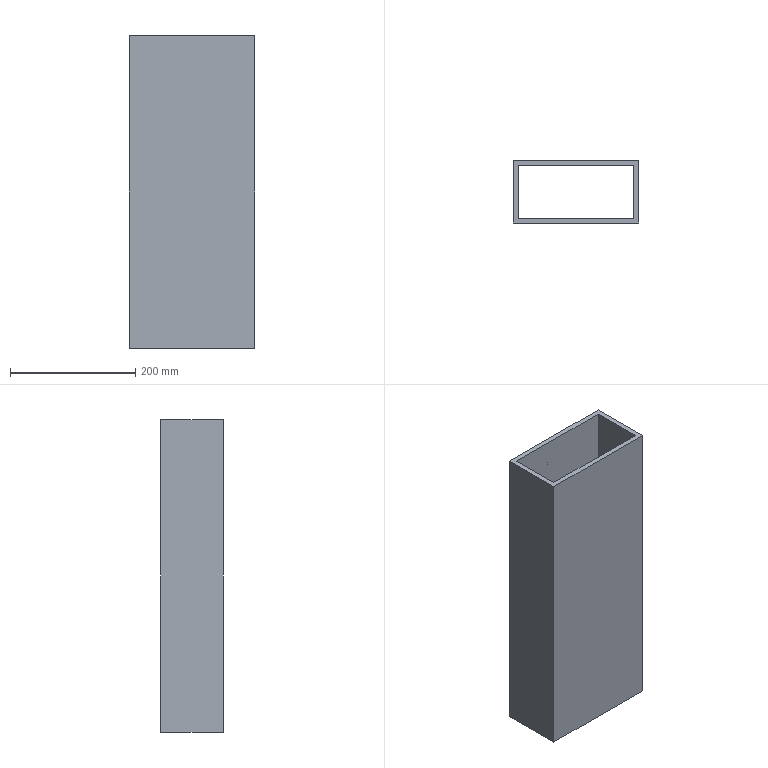Part | SolidWorks | features BaseBody 1 | 1 solid | 34 faces | box 200 x 100 x 500 mm | volume 2270906 mm3 | plane 18 | cylinder 16 | commonest cylinder face diameters 5.3 x16
STEP:
#1=CARTESIAN_POINT('',(20.,43.8,207.35));
#2=VERTEX_POINT('',#1);
#3=CARTESIAN_POINT('',(20.,43.8,212.65));
#4=VERTEX_POINT('',#3);
#5=CARTESIAN_POINT('',(20.,43.8,210.));
#6=DIRECTION('',(0.,1.,0.));
#7=DIRECTION('',(0.,0.,1.));
#8=AXIS2_PLACEMENT_3D('',#5,#6,#7);
#9=CIRCLE('',#8,2.65);
#10=EDGE_CURVE('',#2,#4,#9,.T.);
#11=ORIENTED_EDGE('',*,*,#10,.F.);
#12=CARTESIAN_POINT('',(20.,50.,207.35));
#13=VERTEX_POINT('',#12);
#14=CARTESIAN_POINT('',(20.,43.8,207.35));
#15=DIRECTION('',(0.,1.,0.));
#16=VECTOR('',#15,1000.);
#17=LINE('',#14,#16);
#18=EDGE_CURVE('',#2,#13,#17,.T.);
#19=ORIENTED_EDGE('',*,*,#18,.T.);
#20=CARTESIAN_POINT('',(20.,50.,212.65));
#21=VERTEX_POINT('',#20);
#22=CARTESIAN_POINT('',(20.,50.,210.));
#23=DIRECTION('',(0.,-1.,0.));
#24=DIRECTION('',(0.,0.,1.));
#25=AXIS2_PLACEMENT_3D('',#22,#23,#24);
#26=CIRCLE('',#25,2.65);
#27=EDGE_CURVE('',#21,#13,#26,.T.);
#28=ORIENTED_EDGE('',*,*,#27,.F.);
#29=CARTESIAN_POINT('',(20.,43.8,212.65));
#30=DIRECTION('',(0.,1.,0.));
#31=VECTOR('',#30,1000.);
#32=LINE('',#29,#31);
#33=EDGE_CURVE('',#4,#21,#32,.T.);
#34=ORIENTED_EDGE('',*,*,#33,.F.);
#35=EDGE_LOOP('',(#11,#19,#28,#34));
#36=FACE_OUTER_BOUND('',#35,.T.);
#37=CARTESIAN_POINT('',(20.,43.8,210.));
#38=DIRECTION('',(0.,1.,0.));
#39=DIRECTION('',(0.,0.,1.));
#40=AXIS2_PLACEMENT_3D('',#37,#38,#39);
#41=CYLINDRICAL_SURFACE('',#40,2.65);
#42=ADVANCED_FACE('',(#36),#41,.F.);
#43=CARTESIAN_POINT('',(20.,43.8,87.35));
#44=VERTEX_POINT('',#43);
#45=CARTESIAN_POINT('',(20.,43.8,92.65));
#46=VERTEX_POINT('',#45);
#47=CARTESIAN_POINT('',(20.,43.8,90.));
#48=DIRECTION('',(0.,1.,0.));
#49=DIRECTION('',(0.,0.,1.));
#50=AXIS2_PLACEMENT_3D('',#47,#48,#49);
#51=CIRCLE('',#50,2.65);
#52=EDGE_CURVE('',#44,#46,#51,.T.);
#53=ORIENTED_EDGE('',*,*,#52,.F.);
#54=CARTESIAN_POINT('',(20.,50.,87.35));
#55=VERTEX_POINT('',#54);
#56=CARTESIAN_POINT('',(20.,43.8,87.35));
#57=DIRECTION('',(0.,1.,0.));
#58=VECTOR('',#57,1000.);
#59=LINE('',#56,#58);
#60=EDGE_CURVE('',#44,#55,#59,.T.);
#61=ORIENTED_EDGE('',*,*,#60,.T.);
#62=CARTESIAN_POINT('',(20.,50.,92.65));
#63=VERTEX_POINT('',#62);
#64=CARTESIAN_POINT('',(20.,50.,90.));
#65=DIRECTION('',(0.,-1.,0.));
#66=DIRECTION('',(0.,0.,1.));
#67=AXIS2_PLACEMENT_3D('',#64,#65,#66);
#68=CIRCLE('',#67,2.65);
#69=EDGE_CURVE('',#63,#55,#68,.T.);
#70=ORIENTED_EDGE('',*,*,#69,.F.);
#71=CARTESIAN_POINT('',(20.,43.8,92.65));
#72=DIRECTION('',(0.,1.,0.));
#73=VECTOR('',#72,1000.);
#74=LINE('',#71,#73);
#75=EDGE_CURVE('',#46,#63,#74,.T.);
#76=ORIENTED_EDGE('',*,*,#75,.F.);
#77=EDGE_LOOP('',(#53,#61,#70,#76));
#78=FACE_OUTER_BOUND('',#77,.T.);
#79=CARTESIAN_POINT('',(20.,43.8,90.));
#80=DIRECTION('',(0.,1.,0.));
#81=DIRECTION('',(0.,0.,1.));
#82=AXIS2_PLACEMENT_3D('',#79,#80,#81);
#83=CYLINDRICAL_SURFACE('',#82,2.65);
#84=ADVANCED_FACE('',(#78),#83,.F.);
#85=CARTESIAN_POINT('',(20.,43.8,-32.65));
#86=VERTEX_POINT('',#85);
#87=CARTESIAN_POINT('',(20.,43.8,-27.35));
#88=VERTEX_POINT('',#87);
#89=CARTESIAN_POINT('',(20.,43.8,-30.));
#90=DIRECTION('',(0.,1.,0.));
#91=DIRECTION('',(0.,0.,1.));
#92=AXIS2_PLACEMENT_3D('',#89,#90,#91);
#93=CIRCLE('',#92,2.65);
#94=EDGE_CURVE('',#86,#88,#93,.T.);
#95=ORIENTED_EDGE('',*,*,#94,.F.);
#96=CARTESIAN_POINT('',(20.,50.,-32.65));
#97=VERTEX_POINT('',#96);
#98=CARTESIAN_POINT('',(20.,43.8,-32.65));
#99=DIRECTION('',(0.,1.,0.));
#100=VECTOR('',#99,1000.);
#101=LINE('',#98,#100);
#102=EDGE_CURVE('',#86,#97,#101,.T.);
#103=ORIENTED_EDGE('',*,*,#102,.T.);
#104=CARTESIAN_POINT('',(20.,50.,-27.35));
#105=VERTEX_POINT('',#104);
#106=CARTESIAN_POINT('',(20.,50.,-30.));
#107=DIRECTION('',(0.,-1.,0.));
#108=DIRECTION('',(0.,0.,1.));
#109=AXIS2_PLACEMENT_3D('',#106,#107,#108);
#110=CIRCLE('',#109,2.65);
#111=EDGE_CURVE('',#105,#97,#110,.T.);
#112=ORIENTED_EDGE('',*,*,#111,.F.);
#113=CARTESIAN_POINT('',(20.,43.8,-27.35));
#114=DIRECTION('',(0.,1.,0.));
#115=VECTOR('',#114,1000.);
#116=LINE('',#113,#115);
#117=EDGE_CURVE('',#88,#105,#116,.T.);
#118=ORIENTED_EDGE('',*,*,#117,.F.);
#119=EDGE_LOOP('',(#95,#103,#112,#118));
#120=FACE_OUTER_BOUND('',#119,.T.);
#121=CARTESIAN_POINT('',(20.,43.8,-30.));
#122=DIRECTION('',(0.,1.,0.));
#123=DIRECTION('',(0.,0.,1.));
#124=AXIS2_PLACEMENT_3D('',#121,#122,#123);
#125=CYLINDRICAL_SURFACE('',#124,2.65);
#126=ADVANCED_FACE('',(#120),#125,.F.);
#127=CARTESIAN_POINT('',(20.,43.8,-212.65));
#128=VERTEX_POINT('',#127);
#129=CARTESIAN_POINT('',(20.,43.8,-207.35));
#130=VERTEX_POINT('',#129);
#131=CARTESIAN_POINT('',(20.,43.8,-210.));
#132=DIRECTION('',(0.,1.,0.));
#133=DIRECTION('',(0.,0.,1.));
#134=AXIS2_PLACEMENT_3D('',#131,#132,#133);
#135=CIRCLE('',#134,2.65);
#136=EDGE_CURVE('',#128,#130,#135,.T.);
#137=ORIENTED_EDGE('',*,*,#136,.F.);
#138=CARTESIAN_POINT('',(20.,50.,-212.65));
#139=VERTEX_POINT('',#138);
#140=CARTESIAN_POINT('',(20.,43.8,-212.65));
#141=DIRECTION('',(0.,1.,0.));
#142=VECTOR('',#141,1000.);
#143=LINE('',#140,#142);
#144=EDGE_CURVE('',#128,#139,#143,.T.);
#145=ORIENTED_EDGE('',*,*,#144,.T.);
#146=CARTESIAN_POINT('',(20.,50.,-207.35));
#147=VERTEX_POINT('',#146);
#148=CARTESIAN_POINT('',(20.,50.,-210.));
#149=DIRECTION('',(0.,-1.,0.));
#150=DIRECTION('',(0.,0.,1.));
#151=AXIS2_PLACEMENT_3D('',#148,#149,#150);
#152=CIRCLE('',#151,2.65);
#153=EDGE_CURVE('',#147,#139,#152,.T.);
#154=ORIENTED_EDGE('',*,*,#153,.F.);
#155=CARTESIAN_POINT('',(20.,43.8,-207.35));
#156=DIRECTION('',(0.,1.,0.));
#157=VECTOR('',#156,1000.);
#158=LINE('',#155,#157);
#159=EDGE_CURVE('',#130,#147,#158,.T.);
#160=ORIENTED_EDGE('',*,*,#159,.F.);
#161=EDGE_LOOP('',(#137,#145,#154,#160));
#162=FACE_OUTER_BOUND('',#161,.T.);
#163=CARTESIAN_POINT('',(20.,43.8,-210.));
#164=DIRECTION('',(0.,1.,0.));
#165=DIRECTION('',(0.,0.,1.));
#166=AXIS2_PLACEMENT_3D('',#163,#164,#165);
#167=CYLINDRICAL_SURFACE('',#166,2.65);
#168=ADVANCED_FACE('',(#162),#167,.F.);
#169=CARTESIAN_POINT('',(-20.,43.8,207.35));
#170=VERTEX_POINT('',#169);
#171=CARTESIAN_POINT('',(-20.,43.8,212.65));
#172=VERTEX_POINT('',#171);
#173=CARTESIAN_POINT('',(-20.,43.8,210.));
#174=DIRECTION('',(0.,1.,0.));
#175=DIRECTION('',(0.,0.,1.));
#176=AXIS2_PLACEMENT_3D('',#173,#174,#175);
#177=CIRCLE('',#176,2.65);
#178=EDGE_CURVE('',#170,#172,#177,.T.);
#179=ORIENTED_EDGE('',*,*,#178,.F.);
#180=CARTESIAN_POINT('',(-20.,50.,207.35));
#181=VERTEX_POINT('',#180);
#182=CARTESIAN_POINT('',(-20.,43.8,207.35));
#183=DIRECTION('',(0.,1.,0.));
#184=VECTOR('',#183,1000.);
#185=LINE('',#182,#184);
#186=EDGE_CURVE('',#170,#181,#185,.T.);
#187=ORIENTED_EDGE('',*,*,#186,.T.);
#188=CARTESIAN_POINT('',(-20.,50.,212.65));
#189=VERTEX_POINT('',#188);
#190=CARTESIAN_POINT('',(-20.,50.,210.));
#191=DIRECTION('',(0.,-1.,0.));
#192=DIRECTION('',(0.,0.,1.));
#193=AXIS2_PLACEMENT_3D('',#190,#191,#192);
#194=CIRCLE('',#193,2.65);
#195=EDGE_CURVE('',#189,#181,#194,.T.);
#196=ORIENTED_EDGE('',*,*,#195,.F.);
#197=CARTESIAN_POINT('',(-20.,43.8,212.65));
#198=DIRECTION('',(0.,1.,0.));
#199=VECTOR('',#198,1000.);
#200=LINE('',#197,#199);
#201=EDGE_CURVE('',#172,#189,#200,.T.);
#202=ORIENTED_EDGE('',*,*,#201,.F.);
#203=EDGE_LOOP('',(#179,#187,#196,#202));
#204=FACE_OUTER_BOUND('',#203,.T.);
#205=CARTESIAN_POINT('',(-20.,43.8,210.));
#206=DIRECTION('',(0.,1.,0.));
#207=DIRECTION('',(0.,0.,1.));
#208=AXIS2_PLACEMENT_3D('',#205,#206,#207);
#209=CYLINDRICAL_SURFACE('',#208,2.65);
#210=ADVANCED_FACE('',(#204),#209,.F.);
#211=CARTESIAN_POINT('',(-20.,43.8,87.35));
#212=VERTEX_POINT('',#211);
#213=CARTESIAN_POINT('',(-20.,43.8,92.65));
#214=VERTEX_POINT('',#213);
#215=CARTESIAN_POINT('',(-20.,43.8,90.));
#216=DIRECTION('',(0.,1.,0.));
#217=DIRECTION('',(0.,0.,1.));
#218=AXIS2_PLACEMENT_3D('',#215,#216,#217);
#219=CIRCLE('',#218,2.65);
#220=EDGE_CURVE('',#212,#214,#219,.T.);
#221=ORIENTED_EDGE('',*,*,#220,.F.);
#222=CARTESIAN_POINT('',(-20.,50.,87.35));
#223=VERTEX_POINT('',#222);
#224=CARTESIAN_POINT('',(-20.,43.8,87.35));
#225=DIRECTION('',(0.,1.,0.));
#226=VECTOR('',#225,1000.);
#227=LINE('',#224,#226);
#228=EDGE_CURVE('',#212,#223,#227,.T.);
#229=ORIENTED_EDGE('',*,*,#228,.T.);
#230=CARTESIAN_POINT('',(-20.,50.,92.65));
#231=VERTEX_POINT('',#230);
#232=CARTESIAN_POINT('',(-20.,50.,90.));
#233=DIRECTION('',(0.,-1.,0.));
#234=DIRECTION('',(0.,0.,1.));
#235=AXIS2_PLACEMENT_3D('',#232,#233,#234);
#236=CIRCLE('',#235,2.65);
#237=EDGE_CURVE('',#231,#223,#236,.T.);
#238=ORIENTED_EDGE('',*,*,#237,.F.);
#239=CARTESIAN_POINT('',(-20.,43.8,92.65));
#240=DIRECTION('',(0.,1.,0.));
#241=VECTOR('',#240,1000.);
#242=LINE('',#239,#241);
#243=EDGE_CURVE('',#214,#231,#242,.T.);
#244=ORIENTED_EDGE('',*,*,#243,.F.);
#245=EDGE_LOOP('',(#221,#229,#238,#244));
#246=FACE_OUTER_BOUND('',#245,.T.);
#247=CARTESIAN_POINT('',(-20.,43.8,90.));
#248=DIRECTION('',(0.,1.,0.));
#249=DIRECTION('',(0.,0.,1.));
#250=AXIS2_PLACEMENT_3D('',#247,#248,#249);
#251=CYLINDRICAL_SURFACE('',#250,2.65);
#252=ADVANCED_FACE('',(#246),#251,.F.);
#253=CARTESIAN_POINT('',(-20.,43.8,-32.65));
#254=VERTEX_POINT('',#253);
#255=CARTESIAN_POINT('',(-20.,43.8,-27.35));
#256=VERTEX_POINT('',#255);
#257=CARTESIAN_POINT('',(-20.,43.8,-30.));
#258=DIRECTION('',(0.,1.,0.));
#259=DIRECTION('',(0.,0.,1.));
#260=AXIS2_PLACEMENT_3D('',#257,#258,#259);
#261=CIRCLE('',#260,2.65);
#262=EDGE_CURVE('',#254,#256,#261,.T.);
#263=ORIENTED_EDGE('',*,*,#262,.F.);
#264=CARTESIAN_POINT('',(-20.,50.,-32.65));
#265=VERTEX_POINT('',#264);
#266=CARTESIAN_POINT('',(-20.,43.8,-32.65));
#267=DIRECTION('',(0.,1.,0.));
#268=VECTOR('',#267,1000.);
#269=LINE('',#266,#268);
#270=EDGE_CURVE('',#254,#265,#269,.T.);
#271=ORIENTED_EDGE('',*,*,#270,.T.);
#272=CARTESIAN_POINT('',(-20.,50.,-27.35));
#273=VERTEX_POINT('',#272);
#274=CARTESIAN_POINT('',(-20.,50.,-30.));
#275=DIRECTION('',(0.,-1.,0.));
#276=DIRECTION('',(0.,0.,1.));
#277=AXIS2_PLACEMENT_3D('',#274,#275,#276);
#278=CIRCLE('',#277,2.65);
#279=EDGE_CURVE('',#273,#265,#278,.T.);
#280=ORIENTED_EDGE('',*,*,#279,.F.);
#281=CARTESIAN_POINT('',(-20.,43.8,-27.35));
#282=DIRECTION('',(0.,1.,0.));
#283=VECTOR('',#282,1000.);
#284=LINE('',#281,#283);
#285=EDGE_CURVE('',#256,#273,#284,.T.);
#286=ORIENTED_EDGE('',*,*,#285,.F.);
#287=EDGE_LOOP('',(#263,#271,#280,#286));
#288=FACE_OUTER_BOUND('',#287,.T.);
#289=CARTESIAN_POINT('',(-20.,43.8,-30.));
#290=DIRECTION('',(0.,1.,0.));
#291=DIRECTION('',(0.,0.,1.));
#292=AXIS2_PLACEMENT_3D('',#289,#290,#291);
#293=CYLINDRICAL_SURFACE('',#292,2.65);
#294=ADVANCED_FACE('',(#288),#293,.F.);
#295=CARTESIAN_POINT('',(-20.,43.8,-212.65));
#296=VERTEX_POINT('',#295);
#297=CARTESIAN_POINT('',(-20.,43.8,-207.35));
#298=VERTEX_POINT('',#297);
#299=CARTESIAN_POINT('',(-20.,43.8,-210.));
#300=DIRECTION('',(0.,1.,0.));
#301=DIRECTION('',(0.,0.,1.));
#302=AXIS2_PLACEMENT_3D('',#299,#300,#301);
#303=CIRCLE('',#302,2.65);
#304=EDGE_CURVE('',#296,#298,#303,.T.);
#305=ORIENTED_EDGE('',*,*,#304,.F.);
#306=CARTESIAN_POINT('',(-20.,50.,-212.65));
#307=VERTEX_POINT('',#306);
#308=CARTESIAN_POINT('',(-20.,43.8,-212.65));
#309=DIRECTION('',(0.,1.,0.));
#310=VECTOR('',#309,1000.);
#311=LINE('',#308,#310);
#312=EDGE_CURVE('',#296,#307,#311,.T.);
#313=ORIENTED_EDGE('',*,*,#312,.T.);
#314=CARTESIAN_POINT('',(-20.,50.,-207.35));
#315=VERTEX_POINT('',#314);
#316=CARTESIAN_POINT('',(-20.,50.,-210.));
#317=DIRECTION('',(0.,-1.,0.));
#318=DIRECTION('',(0.,0.,1.));
#319=AXIS2_PLACEMENT_3D('',#316,#317,#318);
#320=CIRCLE('',#319,2.65);
#321=EDGE_CURVE('',#315,#307,#320,.T.);
#322=ORIENTED_EDGE('',*,*,#321,.F.);
#323=CARTESIAN_POINT('',(-20.,43.8,-207.35));
#324=DIRECTION('',(0.,1.,0.));
#325=VECTOR('',#324,1000.);
#326=LINE('',#323,#325);
#327=EDGE_CURVE('',#298,#315,#326,.T.);
#328=ORIENTED_EDGE('',*,*,#327,.F.);
#329=EDGE_LOOP('',(#305,#313,#322,#328));
#330=FACE_OUTER_BOUND('',#329,.T.);
#331=CARTESIAN_POINT('',(-20.,43.8,-210.));
#332=DIRECTION('',(0.,1.,0.));
#333=DIRECTION('',(0.,0.,1.));
#334=AXIS2_PLACEMENT_3D('',#331,#332,#333);
#335=CYLINDRICAL_SURFACE('',#334,2.65);
#336=ADVANCED_FACE('',(#330),#335,.F.);
#337=CARTESIAN_POINT('',(-100.,-50.,250.));
#338=VERTEX_POINT('',#337);
#339=CARTESIAN_POINT('',(100.,-50.,250.));
#340=VERTEX_POINT('',#339);
#341=CARTESIAN_POINT('',(-100.,-50.,250.));
#342=DIRECTION('',(1.,0.,0.));
#343=VECTOR('',#342,1000.);
#344=LINE('',#341,#343);
#345=EDGE_CURVE('',#338,#340,#344,.T.);
#346=ORIENTED_EDGE('',*,*,#345,.F.);
#347=CARTESIAN_POINT('',(-100.,-50.,-250.));
#348=VERTEX_POINT('',#347);
#349=CARTESIAN_POINT('',(-100.,-50.,-250.));
#350=DIRECTION('',(0.,0.,1.));
#351=VECTOR('',#350,1000.);
#352=LINE('',#349,#351);
#353=EDGE_CURVE('',#348,#338,#352,.T.);
#354=ORIENTED_EDGE('',*,*,#353,.F.);
#355=CARTESIAN_POINT('',(100.,-50.,-250.));
#356=VERTEX_POINT('',#355);
#357=CARTESIAN_POINT('',(-100.,-50.,-250.));
#358=DIRECTION('',(-1.,0.,0.));
#359=VECTOR('',#358,1000.);
#360=LINE('',#357,#359);
#361=EDGE_CURVE('',#356,#348,#360,.T.);
#362=ORIENTED_EDGE('',*,*,#361,.F.);
#363=CARTESIAN_POINT('',(100.,-50.,-250.));
#364=DIRECTION('',(0.,0.,-1.));
#365=VECTOR('',#364,1000.);
#366=LINE('',#363,#365);
#367=EDGE_CURVE('',#340,#356,#366,.T.);
#368=ORIENTED_EDGE('',*,*,#367,.F.);
#369=EDGE_LOOP('',(#346,#354,#362,#368));
#370=FACE_OUTER_BOUND('',#369,.T.);
#371=CARTESIAN_POINT('',(-100.,-50.,-250.));
#372=DIRECTION('',(0.,1.,0.));
#373=DIRECTION('',(0.,0.,1.));
#374=AXIS2_PLACEMENT_3D('',#371,#372,#373);
#375=PLANE('',#374);
#376=ADVANCED_FACE('',(#370),#375,.F.);
#377=CARTESIAN_POINT('',(100.,50.,-250.));
#378=VERTEX_POINT('',#377);
#379=CARTESIAN_POINT('',(100.,50.,250.));
#380=VERTEX_POINT('',#379);
#381=CARTESIAN_POINT('',(100.,50.,-250.));
#382=DIRECTION('',(0.,0.,1.));
#383=VECTOR('',#382,1000.);
#384=LINE('',#381,#383);
#385=EDGE_CURVE('',#378,#380,#384,.T.);
#386=ORIENTED_EDGE('',*,*,#385,.T.);
#387=CARTESIAN_POINT('',(100.,-50.,250.));
#388=DIRECTION('',(0.,-1.,0.));
#389=VECTOR('',#388,1000.);
#390=LINE('',#387,#389);
#391=EDGE_CURVE('',#380,#340,#390,.T.);
#392=ORIENTED_EDGE('',*,*,#391,.T.);
#393=ORIENTED_EDGE('',*,*,#367,.T.);
#394=CARTESIAN_POINT('',(100.,-50.,-250.));
#395=DIRECTION('',(0.,1.,0.));
#396=VECTOR('',#395,1000.);
#397=LINE('',#394,#396);
#398=EDGE_CURVE('',#356,#378,#397,.T.);
#399=ORIENTED_EDGE('',*,*,#398,.T.);
#400=EDGE_LOOP('',(#386,#392,#393,#399));
#401=FACE_OUTER_BOUND('',#400,.T.);
#402=CARTESIAN_POINT('',(100.,-50.,-250.));
#403=DIRECTION('',(1.,0.,0.));
#404=DIRECTION('',(0.,0.,-1.));
#405=AXIS2_PLACEMENT_3D('',#402,#403,#404);
#406=PLANE('',#405);
#407=ADVANCED_FACE('',(#401),#406,.T.);
#408=CARTESIAN_POINT('',(-92.,42.,250.));
#409=VERTEX_POINT('',#408);
#410=CARTESIAN_POINT('',(92.,42.,250.));
#411=VERTEX_POINT('',#410);
#412=CARTESIAN_POINT('',(-100.,42.,250.));
#413=DIRECTION('',(1.,0.,0.));
#414=VECTOR('',#413,1000.);
#415=LINE('',#412,#414);
#416=EDGE_CURVE('',#409,#411,#415,.T.);
#417=ORIENTED_EDGE('',*,*,#416,.T.);
#418=CARTESIAN_POINT('',(92.,-42.,250.));
#419=VERTEX_POINT('',#418);
#420=CARTESIAN_POINT('',(92.,-50.,250.));
#421=DIRECTION('',(0.,-1.,0.));
#422=VECTOR('',#421,1000.);
#423=LINE('',#420,#422);
#424=EDGE_CURVE('',#411,#419,#423,.T.);
#425=ORIENTED_EDGE('',*,*,#424,.T.);
#426=CARTESIAN_POINT('',(-92.,-42.,250.));
#427=VERTEX_POINT('',#426);
#428=CARTESIAN_POINT('',(-100.,-42.,250.));
#429=DIRECTION('',(-1.,0.,0.));
#430=VECTOR('',#429,1000.);
#431=LINE('',#428,#430);
#432=EDGE_CURVE('',#419,#427,#431,.T.);
#433=ORIENTED_EDGE('',*,*,#432,.T.);
#434=CARTESIAN_POINT('',(-92.,-50.,250.));
#435=DIRECTION('',(0.,1.,0.));
#436=VECTOR('',#435,1000.);
#437=LINE('',#434,#436);
#438=EDGE_CURVE('',#427,#409,#437,.T.);
#439=ORIENTED_EDGE('',*,*,#438,.T.);
#440=EDGE_LOOP('',(#417,#425,#433,#439));
#441=FACE_BOUND('',#440,.T.);
#442=ORIENTED_EDGE('',*,*,#391,.F.);
#443=CARTESIAN_POINT('',(-100.,50.,250.));
#444=VERTEX_POINT('',#443);
#445=CARTESIAN_POINT('',(-100.,50.,250.));
#446=DIRECTION('',(-1.,0.,0.));
#447=VECTOR('',#446,1000.);
#448=LINE('',#445,#447);
#449=EDGE_CURVE('',#380,#444,#448,.T.);
#450=ORIENTED_EDGE('',*,*,#449,.T.);
#451=CARTESIAN_POINT('',(-100.,-50.,250.));
#452=DIRECTION('',(0.,-1.,0.));
#453=VECTOR('',#452,1000.);
#454=LINE('',#451,#453);
#455=EDGE_CURVE('',#444,#338,#454,.T.);
#456=ORIENTED_EDGE('',*,*,#455,.T.);
#457=ORIENTED_EDGE('',*,*,#345,.T.);
#458=EDGE_LOOP('',(#442,#450,#456,#457));
#459=FACE_OUTER_BOUND('',#458,.T.);
#460=CARTESIAN_POINT('',(-100.,-50.,250.));
#461=DIRECTION('',(0.,0.,1.));
#462=DIRECTION('',(1.,0.,0.));
#463=AXIS2_PLACEMENT_3D('',#460,#461,#462);
#464=PLANE('',#463);
#465=ADVANCED_FACE('',(#441,#459),#464,.T.);
#466=CARTESIAN_POINT('',(-100.,50.,-250.));
#467=VERTEX_POINT('',#466);
#468=CARTESIAN_POINT('',(-100.,50.,-250.));
#469=DIRECTION('',(0.,0.,1.));
#470=VECTOR('',#469,1000.);
#471=LINE('',#468,#470);
#472=EDGE_CURVE('',#467,#444,#471,.T.);
#473=ORIENTED_EDGE('',*,*,#472,.F.);
#474=CARTESIAN_POINT('',(-100.,-50.,-250.));
#475=DIRECTION('',(0.,1.,0.));
#476=VECTOR('',#475,1000.);
#477=LINE('',#474,#476);
#478=EDGE_CURVE('',#348,#467,#477,.T.);
#479=ORIENTED_EDGE('',*,*,#478,.F.);
#480=ORIENTED_EDGE('',*,*,#353,.T.);
#481=ORIENTED_EDGE('',*,*,#455,.F.);
#482=EDGE_LOOP('',(#473,#479,#480,#481));
#483=FACE_OUTER_BOUND('',#482,.T.);
#484=CARTESIAN_POINT('',(-100.,-50.,-250.));
#485=DIRECTION('',(1.,0.,0.));
#486=DIRECTION('',(0.,0.,-1.));
#487=AXIS2_PLACEMENT_3D('',#484,#485,#486);
#488=PLANE('',#487);
#489=ADVANCED_FACE('',(#483),#488,.F.);
#490=CARTESIAN_POINT('',(-92.,42.,-250.));
#491=VERTEX_POINT('',#490);
#492=CARTESIAN_POINT('',(92.,42.,-250.));
#493=VERTEX_POINT('',#492);
#494=CARTESIAN_POINT('',(-100.,42.,-250.));
#495=DIRECTION('',(1.,0.,0.));
#496=VECTOR('',#495,1000.);
#497=LINE('',#494,#496);
#498=EDGE_CURVE('',#491,#493,#497,.T.);
#499=ORIENTED_EDGE('',*,*,#498,.F.);
#500=CARTESIAN_POINT('',(-92.,-42.,-250.));
#501=VERTEX_POINT('',#500);
#502=CARTESIAN_POINT('',(-92.,-50.,-250.));
#503=DIRECTION('',(0.,1.,0.));
#504=VECTOR('',#503,1000.);
#505=LINE('',#502,#504);
#506=EDGE_CURVE('',#501,#491,#505,.T.);
#507=ORIENTED_EDGE('',*,*,#506,.F.);
#508=CARTESIAN_POINT('',(92.,-42.,-250.));
#509=VERTEX_POINT('',#508);
#510=CARTESIAN_POINT('',(-100.,-42.,-250.));
#511=DIRECTION('',(-1.,0.,0.));
#512=VECTOR('',#511,1000.);
#513=LINE('',#510,#512);
#514=EDGE_CURVE('',#509,#501,#513,.T.);
#515=ORIENTED_EDGE('',*,*,#514,.F.);
#516=CARTESIAN_POINT('',(92.,-50.,-250.));
#517=DIRECTION('',(0.,-1.,0.));
#518=VECTOR('',#517,1000.);
#519=LINE('',#516,#518);
#520=EDGE_CURVE('',#493,#509,#519,.T.);
#521=ORIENTED_EDGE('',*,*,#520,.F.);
#522=EDGE_LOOP('',(#499,#507,#515,#521));
#523=FACE_BOUND('',#522,.T.);
#524=ORIENTED_EDGE('',*,*,#398,.F.);
#525=ORIENTED_EDGE('',*,*,#361,.T.);
#526=ORIENTED_EDGE('',*,*,#478,.T.);
#527=CARTESIAN_POINT('',(-100.,50.,-250.));
#528=DIRECTION('',(-1.,0.,0.));
#529=VECTOR('',#528,1000.);
#530=LINE('',#527,#529);
#531=EDGE_CURVE('',#378,#467,#530,.T.);
#532=ORIENTED_EDGE('',*,*,#531,.F.);
#533=EDGE_LOOP('',(#524,#525,#526,#532));
#534=FACE_OUTER_BOUND('',#533,.T.);
#535=CARTESIAN_POINT('',(-100.,-50.,-250.));
#536=DIRECTION('',(0.,0.,1.));
#537=DIRECTION('',(1.,0.,0.));
#538=AXIS2_PLACEMENT_3D('',#535,#536,#537);
#539=PLANE('',#538);
#540=ADVANCED_FACE('',(#523,#534),#539,.F.);
#541=ORIENTED_EDGE('',*,*,#27,.T.);
#542=CARTESIAN_POINT('',(20.,50.,210.));
#543=DIRECTION('',(0.,-1.,0.));
#544=DIRECTION('',(0.,0.,1.));
#545=AXIS2_PLACEMENT_3D('',#542,#543,#544);
#546=CIRCLE('',#545,2.65);
#547=EDGE_CURVE('',#13,#21,#546,.T.);
#548=ORIENTED_EDGE('',*,*,#547,.T.);
#549=EDGE_LOOP('',(#541,#548));
#550=FACE_BOUND('',#549,.T.);
#551=ORIENTED_EDGE('',*,*,#69,.T.);
#552=CARTESIAN_POINT('',(20.,50.,90.));
#553=DIRECTION('',(0.,-1.,0.));
#554=DIRECTION('',(0.,0.,1.));
#555=AXIS2_PLACEMENT_3D('',#552,#553,#554);
#556=CIRCLE('',#555,2.65);
#557=EDGE_CURVE('',#55,#63,#556,.T.);
#558=ORIENTED_EDGE('',*,*,#557,.T.);
#559=EDGE_LOOP('',(#551,#558));
#560=FACE_BOUND('',#559,.T.);
#561=ORIENTED_EDGE('',*,*,#111,.T.);
#562=CARTESIAN_POINT('',(20.,50.,-30.));
#563=DIRECTION('',(0.,-1.,0.));
#564=DIRECTION('',(0.,0.,1.));
#565=AXIS2_PLACEMENT_3D('',#562,#563,#564);
#566=CIRCLE('',#565,2.65);
#567=EDGE_CURVE('',#97,#105,#566,.T.);
#568=ORIENTED_EDGE('',*,*,#567,.T.);
#569=EDGE_LOOP('',(#561,#568));
#570=FACE_BOUND('',#569,.T.);
#571=ORIENTED_EDGE('',*,*,#153,.T.);
#572=CARTESIAN_POINT('',(20.,50.,-210.));
#573=DIRECTION('',(0.,-1.,0.));
#574=DIRECTION('',(0.,0.,1.));
#575=AXIS2_PLACEMENT_3D('',#572,#573,#574);
#576=CIRCLE('',#575,2.65);
#577=EDGE_CURVE('',#139,#147,#576,.T.);
#578=ORIENTED_EDGE('',*,*,#577,.T.);
#579=EDGE_LOOP('',(#571,#578));
#580=FACE_BOUND('',#579,.T.);
#581=ORIENTED_EDGE('',*,*,#195,.T.);
#582=CARTESIAN_POINT('',(-20.,50.,210.));
#583=DIRECTION('',(0.,-1.,0.));
#584=DIRECTION('',(0.,0.,1.));
#585=AXIS2_PLACEMENT_3D('',#582,#583,#584);
#586=CIRCLE('',#585,2.65);
#587=EDGE_CURVE('',#181,#189,#586,.T.);
#588=ORIENTED_EDGE('',*,*,#587,.T.);
#589=EDGE_LOOP('',(#581,#588));
#590=FACE_BOUND('',#589,.T.);
#591=ORIENTED_EDGE('',*,*,#237,.T.);
#592=CARTESIAN_POINT('',(-20.,50.,90.));
#593=DIRECTION('',(0.,-1.,0.));
#594=DIRECTION('',(0.,0.,1.));
#595=AXIS2_PLACEMENT_3D('',#592,#593,#594);
#596=CIRCLE('',#595,2.65);
#597=EDGE_CURVE('',#223,#231,#596,.T.);
#598=ORIENTED_EDGE('',*,*,#597,.T.);
#599=EDGE_LOOP('',(#591,#598));
#600=FACE_BOUND('',#599,.T.);
#601=ORIENTED_EDGE('',*,*,#279,.T.);
#602=CARTESIAN_POINT('',(-20.,50.,-30.));
#603=DIRECTION('',(0.,-1.,0.));
#604=DIRECTION('',(0.,0.,1.));
#605=AXIS2_PLACEMENT_3D('',#602,#603,#604);
#606=CIRCLE('',#605,2.65);
#607=EDGE_CURVE('',#265,#273,#606,.T.);
#608=ORIENTED_EDGE('',*,*,#607,.T.);
#609=EDGE_LOOP('',(#601,#608));
#610=FACE_BOUND('',#609,.T.);
#611=ORIENTED_EDGE('',*,*,#321,.T.);
#612=CARTESIAN_POINT('',(-20.,50.,-210.));
#613=DIRECTION('',(0.,-1.,0.));
#614=DIRECTION('',(0.,0.,1.));
#615=AXIS2_PLACEMENT_3D('',#612,#613,#614);
#616=CIRCLE('',#615,2.65);
#617=EDGE_CURVE('',#307,#315,#616,.T.);
#618=ORIENTED_EDGE('',*,*,#617,.T.);
#619=EDGE_LOOP('',(#611,#618));
#620=FACE_BOUND('',#619,.T.);
#621=ORIENTED_EDGE('',*,*,#449,.F.);
#622=ORIENTED_EDGE('',*,*,#385,.F.);
#623=ORIENTED_EDGE('',*,*,#531,.T.);
#624=ORIENTED_EDGE('',*,*,#472,.T.);
#625=EDGE_LOOP('',(#621,#622,#623,#624));
#626=FACE_OUTER_BOUND('',#625,.T.);
#627=CARTESIAN_POINT('',(-100.,50.,-250.));
#628=DIRECTION('',(0.,1.,0.));
#629=DIRECTION('',(0.,0.,1.));
#630=AXIS2_PLACEMENT_3D('',#627,#628,#629);
#631=PLANE('',#630);
#632=ADVANCED_FACE('',(#550,#560,#570,#580,#590,#600,#610,#620,#626),#631,.T.);
#633=CARTESIAN_POINT('',(92.,42.,-251.));
#634=DIRECTION('',(0.,0.,1.));
#635=VECTOR('',#634,1000.);
#636=LINE('',#633,#635);
#637=EDGE_CURVE('',#493,#411,#636,.T.);
#638=ORIENTED_EDGE('',*,*,#637,.F.);
#639=ORIENTED_EDGE('',*,*,#520,.T.);
#640=CARTESIAN_POINT('',(92.,-42.,-251.));
#641=DIRECTION('',(0.,0.,-1.));
#642=VECTOR('',#641,1000.);
#643=LINE('',#640,#642);
#644=EDGE_CURVE('',#419,#509,#643,.T.);
#645=ORIENTED_EDGE('',*,*,#644,.F.);
#646=ORIENTED_EDGE('',*,*,#424,.F.);
#647=EDGE_LOOP('',(#638,#639,#645,#646));
#648=FACE_OUTER_BOUND('',#647,.T.);
#649=CARTESIAN_POINT('',(92.,-42.,-251.));
#650=DIRECTION('',(1.,0.,0.));
#651=DIRECTION('',(0.,0.,-1.));
#652=AXIS2_PLACEMENT_3D('',#649,#650,#651);
#653=PLANE('',#652);
#654=ADVANCED_FACE('',(#648),#653,.F.);
#655=CARTESIAN_POINT('',(-92.,42.,-251.));
#656=DIRECTION('',(0.,0.,1.));
#657=VECTOR('',#656,1000.);
#658=LINE('',#655,#657);
#659=EDGE_CURVE('',#491,#409,#658,.T.);
#660=ORIENTED_EDGE('',*,*,#659,.F.);
#661=ORIENTED_EDGE('',*,*,#498,.T.);
#662=ORIENTED_EDGE('',*,*,#637,.T.);
#663=ORIENTED_EDGE('',*,*,#416,.F.);
#664=EDGE_LOOP('',(#660,#661,#662,#663));
#665=FACE_OUTER_BOUND('',#664,.T.);
#666=CARTESIAN_POINT('',(-92.,42.,-251.));
#667=DIRECTION('',(0.,1.,0.));
#668=DIRECTION('',(0.,0.,1.));
#669=AXIS2_PLACEMENT_3D('',#666,#667,#668);
#670=PLANE('',#669);
#671=ADVANCED_FACE('',(#665),#670,.F.);
#672=ORIENTED_EDGE('',*,*,#659,.T.);
#673=ORIENTED_EDGE('',*,*,#438,.F.);
#674=CARTESIAN_POINT('',(-92.,-42.,-251.));
#675=DIRECTION('',(0.,0.,-1.));
#676=VECTOR('',#675,1000.);
#677=LINE('',#674,#676);
#678=EDGE_CURVE('',#427,#501,#677,.T.);
#679=ORIENTED_EDGE('',*,*,#678,.T.);
#680=ORIENTED_EDGE('',*,*,#506,.T.);
#681=EDGE_LOOP('',(#672,#673,#679,#680));
#682=FACE_OUTER_BOUND('',#681,.T.);
#683=CARTESIAN_POINT('',(-92.,-42.,-251.));
#684=DIRECTION('',(1.,0.,0.));
#685=DIRECTION('',(0.,0.,-1.));
#686=AXIS2_PLACEMENT_3D('',#683,#684,#685);
#687=PLANE('',#686);
#688=ADVANCED_FACE('',(#682),#687,.T.);
#689=ORIENTED_EDGE('',*,*,#678,.F.);
#690=ORIENTED_EDGE('',*,*,#432,.F.);
#691=ORIENTED_EDGE('',*,*,#644,.T.);
#692=ORIENTED_EDGE('',*,*,#514,.T.);
#693=EDGE_LOOP('',(#689,#690,#691,#692));
#694=FACE_OUTER_BOUND('',#693,.T.);
#695=CARTESIAN_POINT('',(-92.,-42.,-251.));
#696=DIRECTION('',(0.,1.,0.));
#697=DIRECTION('',(0.,0.,1.));
#698=AXIS2_PLACEMENT_3D('',#695,#696,#697);
#699=PLANE('',#698);
#700=ADVANCED_FACE('',(#694),#699,.T.);
#701=ORIENTED_EDGE('',*,*,#18,.F.);
#702=CARTESIAN_POINT('',(20.,43.8,210.));
#703=DIRECTION('',(0.,1.,0.));
#704=DIRECTION('',(0.,0.,1.));
#705=AXIS2_PLACEMENT_3D('',#702,#703,#704);
#706=CIRCLE('',#705,2.65);
#707=EDGE_CURVE('',#4,#2,#706,.T.);
#708=ORIENTED_EDGE('',*,*,#707,.F.);
#709=ORIENTED_EDGE('',*,*,#33,.T.);
#710=ORIENTED_EDGE('',*,*,#547,.F.);
#711=EDGE_LOOP('',(#701,#708,#709,#710));
#712=FACE_OUTER_BOUND('',#711,.T.);
#713=CARTESIAN_POINT('',(20.,43.8,210.));
#714=DIRECTION('',(0.,1.,0.));
#715=DIRECTION('',(0.,0.,1.));
#716=AXIS2_PLACEMENT_3D('',#713,#714,#715);
#717=CYLINDRICAL_SURFACE('',#716,2.65);
#718=ADVANCED_FACE('',(#712),#717,.F.);
#719=ORIENTED_EDGE('',*,*,#60,.F.);
#720=CARTESIAN_POINT('',(20.,43.8,90.));
#721=DIRECTION('',(0.,1.,0.));
#722=DIRECTION('',(0.,0.,1.));
#723=AXIS2_PLACEMENT_3D('',#720,#721,#722);
#724=CIRCLE('',#723,2.65);
#725=EDGE_CURVE('',#46,#44,#724,.T.);
#726=ORIENTED_EDGE('',*,*,#725,.F.);
#727=ORIENTED_EDGE('',*,*,#75,.T.);
#728=ORIENTED_EDGE('',*,*,#557,.F.);
#729=EDGE_LOOP('',(#719,#726,#727,#728));
#730=FACE_OUTER_BOUND('',#729,.T.);
#731=CARTESIAN_POINT('',(20.,43.8,90.));
#732=DIRECTION('',(0.,1.,0.));
#733=DIRECTION('',(0.,0.,1.));
#734=AXIS2_PLACEMENT_3D('',#731,#732,#733);
#735=CYLINDRICAL_SURFACE('',#734,2.65);
#736=ADVANCED_FACE('',(#730),#735,.F.);
#737=ORIENTED_EDGE('',*,*,#102,.F.);
#738=CARTESIAN_POINT('',(20.,43.8,-30.));
#739=DIRECTION('',(0.,1.,0.));
#740=DIRECTION('',(0.,0.,1.));
#741=AXIS2_PLACEMENT_3D('',#738,#739,#740);
#742=CIRCLE('',#741,2.65);
#743=EDGE_CURVE('',#88,#86,#742,.T.);
#744=ORIENTED_EDGE('',*,*,#743,.F.);
#745=ORIENTED_EDGE('',*,*,#117,.T.);
#746=ORIENTED_EDGE('',*,*,#567,.F.);
#747=EDGE_LOOP('',(#737,#744,#745,#746));
#748=FACE_OUTER_BOUND('',#747,.T.);
#749=CARTESIAN_POINT('',(20.,43.8,-30.));
#750=DIRECTION('',(0.,1.,0.));
#751=DIRECTION('',(0.,0.,1.));
#752=AXIS2_PLACEMENT_3D('',#749,#750,#751);
#753=CYLINDRICAL_SURFACE('',#752,2.65);
#754=ADVANCED_FACE('',(#748),#753,.F.);
#755=ORIENTED_EDGE('',*,*,#144,.F.);
#756=CARTESIAN_POINT('',(20.,43.8,-210.));
#757=DIRECTION('',(0.,1.,0.));
#758=DIRECTION('',(0.,0.,1.));
#759=AXIS2_PLACEMENT_3D('',#756,#757,#758);
#760=CIRCLE('',#759,2.65);
#761=EDGE_CURVE('',#130,#128,#760,.T.);
#762=ORIENTED_EDGE('',*,*,#761,.F.);
#763=ORIENTED_EDGE('',*,*,#159,.T.);
#764=ORIENTED_EDGE('',*,*,#577,.F.);
#765=EDGE_LOOP('',(#755,#762,#763,#764));
#766=FACE_OUTER_BOUND('',#765,.T.);
#767=CARTESIAN_POINT('',(20.,43.8,-210.));
#768=DIRECTION('',(0.,1.,0.));
#769=DIRECTION('',(0.,0.,1.));
#770=AXIS2_PLACEMENT_3D('',#767,#768,#769);
#771=CYLINDRICAL_SURFACE('',#770,2.65);
#772=ADVANCED_FACE('',(#766),#771,.F.);
#773=ORIENTED_EDGE('',*,*,#186,.F.);
#774=CARTESIAN_POINT('',(-20.,43.8,210.));
#775=DIRECTION('',(0.,1.,0.));
#776=DIRECTION('',(0.,0.,1.));
#777=AXIS2_PLACEMENT_3D('',#774,#775,#776);
#778=CIRCLE('',#777,2.65);
#779=EDGE_CURVE('',#172,#170,#778,.T.);
#780=ORIENTED_EDGE('',*,*,#779,.F.);
#781=ORIENTED_EDGE('',*,*,#201,.T.);
#782=ORIENTED_EDGE('',*,*,#587,.F.);
#783=EDGE_LOOP('',(#773,#780,#781,#782));
#784=FACE_OUTER_BOUND('',#783,.T.);
#785=CARTESIAN_POINT('',(-20.,43.8,210.));
#786=DIRECTION('',(0.,1.,0.));
#787=DIRECTION('',(0.,0.,1.));
#788=AXIS2_PLACEMENT_3D('',#785,#786,#787);
#789=CYLINDRICAL_SURFACE('',#788,2.65);
#790=ADVANCED_FACE('',(#784),#789,.F.);
#791=ORIENTED_EDGE('',*,*,#228,.F.);
#792=CARTESIAN_POINT('',(-20.,43.8,90.));
#793=DIRECTION('',(0.,1.,0.));
#794=DIRECTION('',(0.,0.,1.));
#795=AXIS2_PLACEMENT_3D('',#792,#793,#794);
#796=CIRCLE('',#795,2.65);
#797=EDGE_CURVE('',#214,#212,#796,.T.);
#798=ORIENTED_EDGE('',*,*,#797,.F.);
#799=ORIENTED_EDGE('',*,*,#243,.T.);
#800=ORIENTED_EDGE('',*,*,#597,.F.);
#801=EDGE_LOOP('',(#791,#798,#799,#800));
#802=FACE_OUTER_BOUND('',#801,.T.);
#803=CARTESIAN_POINT('',(-20.,43.8,90.));
#804=DIRECTION('',(0.,1.,0.));
#805=DIRECTION('',(0.,0.,1.));
#806=AXIS2_PLACEMENT_3D('',#803,#804,#805);
#807=CYLINDRICAL_SURFACE('',#806,2.65);
#808=ADVANCED_FACE('',(#802),#807,.F.);
#809=ORIENTED_EDGE('',*,*,#270,.F.);
#810=CARTESIAN_POINT('',(-20.,43.8,-30.));
#811=DIRECTION('',(0.,1.,0.));
#812=DIRECTION('',(0.,0.,1.));
#813=AXIS2_PLACEMENT_3D('',#810,#811,#812);
#814=CIRCLE('',#813,2.65);
#815=EDGE_CURVE('',#256,#254,#814,.T.);
#816=ORIENTED_EDGE('',*,*,#815,.F.);
#817=ORIENTED_EDGE('',*,*,#285,.T.);
#818=ORIENTED_EDGE('',*,*,#607,.F.);
#819=EDGE_LOOP('',(#809,#816,#817,#818));
#820=FACE_OUTER_BOUND('',#819,.T.);
#821=CARTESIAN_POINT('',(-20.,43.8,-30.));
#822=DIRECTION('',(0.,1.,0.));
#823=DIRECTION('',(0.,0.,1.));
#824=AXIS2_PLACEMENT_3D('',#821,#822,#823);
#825=CYLINDRICAL_SURFACE('',#824,2.65);
#826=ADVANCED_FACE('',(#820),#825,.F.);
#827=ORIENTED_EDGE('',*,*,#312,.F.);
#828=CARTESIAN_POINT('',(-20.,43.8,-210.));
#829=DIRECTION('',(0.,1.,0.));
#830=DIRECTION('',(0.,0.,1.));
#831=AXIS2_PLACEMENT_3D('',#828,#829,#830);
#832=CIRCLE('',#831,2.65);
#833=EDGE_CURVE('',#298,#296,#832,.T.);
#834=ORIENTED_EDGE('',*,*,#833,.F.);
#835=ORIENTED_EDGE('',*,*,#327,.T.);
#836=ORIENTED_EDGE('',*,*,#617,.F.);
#837=EDGE_LOOP('',(#827,#834,#835,#836));
#838=FACE_OUTER_BOUND('',#837,.T.);
#839=CARTESIAN_POINT('',(-20.,43.8,-210.));
#840=DIRECTION('',(0.,1.,0.));
#841=DIRECTION('',(0.,0.,1.));
#842=AXIS2_PLACEMENT_3D('',#839,#840,#841);
#843=CYLINDRICAL_SURFACE('',#842,2.65);
#844=ADVANCED_FACE('',(#838),#843,.F.);
#845=ORIENTED_EDGE('',*,*,#707,.T.);
#846=ORIENTED_EDGE('',*,*,#10,.T.);
#847=EDGE_LOOP('',(#845,#846));
#848=FACE_OUTER_BOUND('',#847,.T.);
#849=CARTESIAN_POINT('',(20.,43.8,210.));
#850=DIRECTION('',(0.,1.,0.));
#851=DIRECTION('',(0.,0.,1.));
#852=AXIS2_PLACEMENT_3D('',#849,#850,#851);
#853=PLANE('',#852);
#854=ADVANCED_FACE('',(#848),#853,.T.);
#855=ORIENTED_EDGE('',*,*,#725,.T.);
#856=ORIENTED_EDGE('',*,*,#52,.T.);
#857=EDGE_LOOP('',(#855,#856));
#858=FACE_OUTER_BOUND('',#857,.T.);
#859=CARTESIAN_POINT('',(20.,43.8,90.));
#860=DIRECTION('',(0.,1.,0.));
#861=DIRECTION('',(0.,0.,1.));
#862=AXIS2_PLACEMENT_3D('',#859,#860,#861);
#863=PLANE('',#862);
#864=ADVANCED_FACE('',(#858),#863,.T.);
#865=ORIENTED_EDGE('',*,*,#743,.T.);
#866=ORIENTED_EDGE('',*,*,#94,.T.);
#867=EDGE_LOOP('',(#865,#866));
#868=FACE_OUTER_BOUND('',#867,.T.);
#869=CARTESIAN_POINT('',(20.,43.8,-30.));
#870=DIRECTION('',(0.,1.,0.));
#871=DIRECTION('',(0.,0.,1.));
#872=AXIS2_PLACEMENT_3D('',#869,#870,#871);
#873=PLANE('',#872);
#874=ADVANCED_FACE('',(#868),#873,.T.);
#875=ORIENTED_EDGE('',*,*,#761,.T.);
#876=ORIENTED_EDGE('',*,*,#136,.T.);
#877=EDGE_LOOP('',(#875,#876));
#878=FACE_OUTER_BOUND('',#877,.T.);
#879=CARTESIAN_POINT('',(20.,43.8,-210.));
#880=DIRECTION('',(0.,1.,0.));
#881=DIRECTION('',(0.,0.,1.));
#882=AXIS2_PLACEMENT_3D('',#879,#880,#881);
#883=PLANE('',#882);
#884=ADVANCED_FACE('',(#878),#883,.T.);
#885=ORIENTED_EDGE('',*,*,#779,.T.);
#886=ORIENTED_EDGE('',*,*,#178,.T.);
#887=EDGE_LOOP('',(#885,#886));
#888=FACE_OUTER_BOUND('',#887,.T.);
#889=CARTESIAN_POINT('',(-20.,43.8,210.));
#890=DIRECTION('',(0.,1.,0.));
#891=DIRECTION('',(0.,0.,1.));
#892=AXIS2_PLACEMENT_3D('',#889,#890,#891);
#893=PLANE('',#892);
#894=ADVANCED_FACE('',(#888),#893,.T.);
#895=ORIENTED_EDGE('',*,*,#797,.T.);
#896=ORIENTED_EDGE('',*,*,#220,.T.);
#897=EDGE_LOOP('',(#895,#896));
#898=FACE_OUTER_BOUND('',#897,.T.);
#899=CARTESIAN_POINT('',(-20.,43.8,90.));
#900=DIRECTION('',(0.,1.,0.));
#901=DIRECTION('',(0.,0.,1.));
#902=AXIS2_PLACEMENT_3D('',#899,#900,#901);
#903=PLANE('',#902);
#904=ADVANCED_FACE('',(#898),#903,.T.);
#905=ORIENTED_EDGE('',*,*,#815,.T.);
#906=ORIENTED_EDGE('',*,*,#262,.T.);
#907=EDGE_LOOP('',(#905,#906));
#908=FACE_OUTER_BOUND('',#907,.T.);
#909=CARTESIAN_POINT('',(-20.,43.8,-30.));
#910=DIRECTION('',(0.,1.,0.));
#911=DIRECTION('',(0.,0.,1.));
#912=AXIS2_PLACEMENT_3D('',#909,#910,#911);
#913=PLANE('',#912);
#914=ADVANCED_FACE('',(#908),#913,.T.);
#915=ORIENTED_EDGE('',*,*,#833,.T.);
#916=ORIENTED_EDGE('',*,*,#304,.T.);
#917=EDGE_LOOP('',(#915,#916));
#918=FACE_OUTER_BOUND('',#917,.T.);
#919=CARTESIAN_POINT('',(-20.,43.8,-210.));
#920=DIRECTION('',(0.,1.,0.));
#921=DIRECTION('',(0.,0.,1.));
#922=AXIS2_PLACEMENT_3D('',#919,#920,#921);
#923=PLANE('',#922);
#924=ADVANCED_FACE('',(#918),#923,.T.);
#925=CLOSED_SHELL('',(#42,#84,#126,#168,#210,#252,#294,#336,#376,#407,#465,#489,#540,#632,#654,#671,#688,#700,#718,#736,#754,#772,#790,#808,#826,#844,#854,#864,#874,#884,#894,#904,#914,#924));
#926=MANIFOLD_SOLID_BREP('',#925);
#927=CARTESIAN_POINT('',(0.,0.,0.));
#928=DIRECTION('',(0.,0.,1.));
#929=DIRECTION('',(1.,0.,0.));
#930=AXIS2_PLACEMENT_3D('',#927,#928,#929);
#931=(LENGTH_UNIT()NAMED_UNIT(*)SI_UNIT(.MILLI.,.METRE.));
#932=UNCERTAINTY_MEASURE_WITH_UNIT(LENGTH_MEASURE(0.00001),#931,'','');
#933=(NAMED_UNIT(*)PLANE_ANGLE_UNIT()SI_UNIT($,.RADIAN.));
#934=(NAMED_UNIT(*)SI_UNIT($,.STERADIAN.)SOLID_ANGLE_UNIT());
#935=(GEOMETRIC_REPRESENTATION_CONTEXT(3)GLOBAL_UNCERTAINTY_ASSIGNED_CONTEXT((#932))GLOBAL_UNIT_ASSIGNED_CONTEXT((#931,#933,#934))REPRESENTATION_CONTEXT('',''));
#936=ADVANCED_BREP_SHAPE_REPRESENTATION('',(#926,#930),#935);